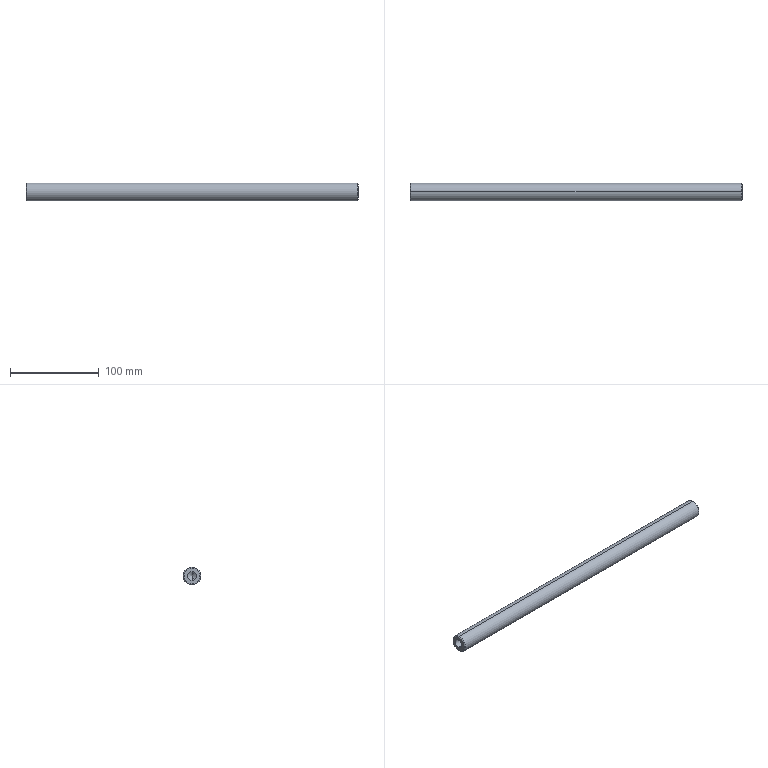Part | STEP file | BU-A02a | 1 solid | 16 faces | box 375 x 20 x 20 mm | volume 113660 mm3 | cone 8 | cylinder 6 | plane 2 | commonest cylinder face diameters 10.2 x4 20 x2
STEP:
#1=CARTESIAN_POINT('',(0.,0.,0.));
#2=DIRECTION('',(0.,0.,1.));
#3=DIRECTION('',(1.,0.,0.));
#4=AXIS2_PLACEMENT_3D('',#1,#2,#3);
#5=CARTESIAN_POINT('',(375.,0.,-9.));
#6=VERTEX_POINT('',#5);
#7=CARTESIAN_POINT('',(375.,0.,9.));
#8=VERTEX_POINT('',#7);
#9=CARTESIAN_POINT('',(375.,0.,0.));
#10=DIRECTION('',(1.,0.,0.));
#11=DIRECTION('',(0.,0.,1.));
#12=AXIS2_PLACEMENT_3D('',#9,#10,#11);
#13=CIRCLE('',#12,9.);
#14=CARTESIAN_POINT('',(374.,0.,0.));
#15=DIRECTION('',(-1.,0.,0.));
#16=DIRECTION('',(0.,0.,1.));
#17=AXIS2_PLACEMENT_3D('',#14,#15,#16);
#18=CONICAL_SURFACE('',#17,10.,0.7854);
#19=CARTESIAN_POINT('',(6.283,-1.));
#20=DIRECTION('',(-1.,0.));
#21=VECTOR('',#20,1.);
#22=LINE('',#19,#21);
#23=(GEOMETRIC_REPRESENTATION_CONTEXT(2)PARAMETRIC_REPRESENTATION_CONTEXT()REPRESENTATION_CONTEXT('',''));
#24=DEFINITIONAL_REPRESENTATION('',(#22),#23);
#25=PCURVE('',#18,#24);
#26=CARTESIAN_POINT('',(375.,0.,0.));
#27=DIRECTION('',(-1.,0.,0.));
#28=DIRECTION('',(0.,0.,1.));
#29=AXIS2_PLACEMENT_3D('',#26,#27,#28);
#30=PLANE('',#29);
#31=CARTESIAN_POINT('',(9.,0.));
#32=CARTESIAN_POINT('',(9.,-15.588));
#33=CARTESIAN_POINT('',(-4.5,-7.794));
#34=CARTESIAN_POINT('',(-18.,0.));
#35=CARTESIAN_POINT('',(-4.5,7.794));
#36=CARTESIAN_POINT('',(9.,15.588));
#37=CARTESIAN_POINT('',(9.,0.));
#38=(BOUNDED_CURVE()B_SPLINE_CURVE(2,(#31,#32,#33,#34,#35,#36,#37),.UNSPECIFIED.,.T.,.F.)B_SPLINE_CURVE_WITH_KNOTS((1,2,2,2,2,1),(-2.094,0.,2.094,4.189,6.283,8.378),.UNSPECIFIED.)CURVE()GEOMETRIC_REPRESENTATION_ITEM()RATIONAL_B_SPLINE_CURVE((1.,0.5,1.,0.5,1.,0.5,1.))REPRESENTATION_ITEM(''));
#39=(GEOMETRIC_REPRESENTATION_CONTEXT(2)PARAMETRIC_REPRESENTATION_CONTEXT()REPRESENTATION_CONTEXT('',''));
#40=DEFINITIONAL_REPRESENTATION('',(#38),#39);
#41=PCURVE('',#30,#40);
#42=SURFACE_CURVE('',#13,(#25,#41),.PCURVE_S1.);
#43=EDGE_CURVE('',#6,#8,#42,.T.);
#44=ORIENTED_EDGE('',*,*,#43,.F.);
#45=CARTESIAN_POINT('',(374.,0.,-10.));
#46=VERTEX_POINT('',#45);
#47=CARTESIAN_POINT('',(374.,0.,-10.));
#48=DIRECTION('',(-0.7071,0.,-0.7071));
#49=VECTOR('',#48,1.);
#50=LINE('',#47,#49);
#51=CARTESIAN_POINT('',(3.142,0.));
#52=DIRECTION('',(0.,1.));
#53=VECTOR('',#52,1.);
#54=LINE('',#51,#53);
#55=(GEOMETRIC_REPRESENTATION_CONTEXT(2)PARAMETRIC_REPRESENTATION_CONTEXT()REPRESENTATION_CONTEXT('',''));
#56=DEFINITIONAL_REPRESENTATION('',(#54),#55);
#57=PCURVE('',#18,#56);
#58=CARTESIAN_POINT('',(374.,0.,0.));
#59=DIRECTION('',(-1.,0.,0.));
#60=DIRECTION('',(0.,0.,1.));
#61=AXIS2_PLACEMENT_3D('',#58,#59,#60);
#62=CONICAL_SURFACE('',#61,10.,0.7854);
#63=CARTESIAN_POINT('',(3.142,0.));
#64=DIRECTION('',(0.,1.));
#65=VECTOR('',#64,1.);
#66=LINE('',#63,#65);
#67=(GEOMETRIC_REPRESENTATION_CONTEXT(2)PARAMETRIC_REPRESENTATION_CONTEXT()REPRESENTATION_CONTEXT('',''));
#68=DEFINITIONAL_REPRESENTATION('',(#66),#67);
#69=PCURVE('',#62,#68);
#70=SURFACE_CURVE('',#50,(#57,#69),.PCURVE_S1.);
#71=EDGE_CURVE('',#6,#46,#70,.T.);
#72=ORIENTED_EDGE('',*,*,#71,.T.);
#73=CARTESIAN_POINT('',(374.,0.,10.));
#74=VERTEX_POINT('',#73);
#75=CARTESIAN_POINT('',(374.,0.,0.));
#76=DIRECTION('',(-1.,0.,0.));
#77=DIRECTION('',(0.,0.,1.));
#78=AXIS2_PLACEMENT_3D('',#75,#76,#77);
#79=CIRCLE('',#78,10.);
#80=CARTESIAN_POINT('',(0.,0.));
#81=DIRECTION('',(1.,0.));
#82=VECTOR('',#81,1.);
#83=LINE('',#80,#82);
#84=(GEOMETRIC_REPRESENTATION_CONTEXT(2)PARAMETRIC_REPRESENTATION_CONTEXT()REPRESENTATION_CONTEXT('',''));
#85=DEFINITIONAL_REPRESENTATION('',(#83),#84);
#86=PCURVE('',#18,#85);
#87=CARTESIAN_POINT('',(-1000.,0.,0.));
#88=DIRECTION('',(-1.,0.,0.));
#89=DIRECTION('',(0.,0.,1.));
#90=AXIS2_PLACEMENT_3D('',#87,#88,#89);
#91=CYLINDRICAL_SURFACE('',#90,10.);
#92=CARTESIAN_POINT('',(0.,-1374.));
#93=DIRECTION('',(1.,0.));
#94=VECTOR('',#93,1.);
#95=LINE('',#92,#94);
#96=(GEOMETRIC_REPRESENTATION_CONTEXT(2)PARAMETRIC_REPRESENTATION_CONTEXT()REPRESENTATION_CONTEXT('',''));
#97=DEFINITIONAL_REPRESENTATION('',(#95),#96);
#98=PCURVE('',#91,#97);
#99=SURFACE_CURVE('',#79,(#86,#98),.PCURVE_S1.);
#100=EDGE_CURVE('',#74,#46,#99,.T.);
#101=ORIENTED_EDGE('',*,*,#100,.F.);
#102=CARTESIAN_POINT('',(374.,0.,10.));
#103=DIRECTION('',(-0.7071,0.,0.7071));
#104=VECTOR('',#103,1.);
#105=LINE('',#102,#104);
#106=CARTESIAN_POINT('',(0.,0.));
#107=DIRECTION('',(0.,1.));
#108=VECTOR('',#107,1.);
#109=LINE('',#106,#108);
#110=(GEOMETRIC_REPRESENTATION_CONTEXT(2)PARAMETRIC_REPRESENTATION_CONTEXT()REPRESENTATION_CONTEXT('',''));
#111=DEFINITIONAL_REPRESENTATION('',(#109),#110);
#112=PCURVE('',#18,#111);
#113=CARTESIAN_POINT('',(6.283,0.));
#114=DIRECTION('',(0.,1.));
#115=VECTOR('',#114,1.);
#116=LINE('',#113,#115);
#117=(GEOMETRIC_REPRESENTATION_CONTEXT(2)PARAMETRIC_REPRESENTATION_CONTEXT()REPRESENTATION_CONTEXT('',''));
#118=DEFINITIONAL_REPRESENTATION('',(#116),#117);
#119=PCURVE('',#62,#118);
#120=SURFACE_CURVE('',#105,(#112,#119),.PCURVE_S1.);
#121=EDGE_CURVE('',#8,#74,#120,.T.);
#122=ORIENTED_EDGE('',*,*,#121,.F.);
#123=EDGE_LOOP('',(#44,#72,#101,#122));
#124=FACE_BOUND('',#123,.T.);
#125=ADVANCED_FACE('',(#124),#18,.T.);
#126=CARTESIAN_POINT('',(0.,0.,9.));
#127=VERTEX_POINT('',#126);
#128=CARTESIAN_POINT('',(0.,0.,-9.));
#129=VERTEX_POINT('',#128);
#130=CARTESIAN_POINT('',(0.,0.,0.));
#131=DIRECTION('',(-1.,0.,0.));
#132=DIRECTION('',(0.,0.,-1.));
#133=AXIS2_PLACEMENT_3D('',#130,#131,#132);
#134=CIRCLE('',#133,9.);
#135=CARTESIAN_POINT('',(0.,0.,0.));
#136=DIRECTION('',(1.,0.,0.));
#137=DIRECTION('',(0.,0.,-1.));
#138=AXIS2_PLACEMENT_3D('',#135,#136,#137);
#139=CONICAL_SURFACE('',#138,9.,0.7854);
#140=CARTESIAN_POINT('',(6.283,0.));
#141=DIRECTION('',(-1.,0.));
#142=VECTOR('',#141,1.);
#143=LINE('',#140,#142);
#144=(GEOMETRIC_REPRESENTATION_CONTEXT(2)PARAMETRIC_REPRESENTATION_CONTEXT()REPRESENTATION_CONTEXT('',''));
#145=DEFINITIONAL_REPRESENTATION('',(#143),#144);
#146=PCURVE('',#139,#145);
#147=CARTESIAN_POINT('',(0.,0.,0.));
#148=DIRECTION('',(1.,0.,0.));
#149=DIRECTION('',(0.,0.,-1.));
#150=AXIS2_PLACEMENT_3D('',#147,#148,#149);
#151=PLANE('',#150);
#152=CARTESIAN_POINT('',(9.,0.));
#153=CARTESIAN_POINT('',(9.,-15.588));
#154=CARTESIAN_POINT('',(-4.5,-7.794));
#155=CARTESIAN_POINT('',(-18.,0.));
#156=CARTESIAN_POINT('',(-4.5,7.794));
#157=CARTESIAN_POINT('',(9.,15.588));
#158=CARTESIAN_POINT('',(9.,0.));
#159=(BOUNDED_CURVE()B_SPLINE_CURVE(2,(#152,#153,#154,#155,#156,#157,#158),.UNSPECIFIED.,.T.,.F.)B_SPLINE_CURVE_WITH_KNOTS((1,2,2,2,2,1),(-2.094,0.,2.094,4.189,6.283,8.378),.UNSPECIFIED.)CURVE()GEOMETRIC_REPRESENTATION_ITEM()RATIONAL_B_SPLINE_CURVE((1.,0.5,1.,0.5,1.,0.5,1.))REPRESENTATION_ITEM(''));
#160=(GEOMETRIC_REPRESENTATION_CONTEXT(2)PARAMETRIC_REPRESENTATION_CONTEXT()REPRESENTATION_CONTEXT('',''));
#161=DEFINITIONAL_REPRESENTATION('',(#159),#160);
#162=PCURVE('',#151,#161);
#163=SURFACE_CURVE('',#134,(#146,#162),.PCURVE_S1.);
#164=EDGE_CURVE('',#127,#129,#163,.T.);
#165=ORIENTED_EDGE('',*,*,#164,.F.);
#166=CARTESIAN_POINT('',(1.,0.,10.));
#167=VERTEX_POINT('',#166);
#168=CARTESIAN_POINT('',(0.,0.,9.));
#169=DIRECTION('',(0.7071,0.,0.7071));
#170=VECTOR('',#169,1.);
#171=LINE('',#168,#170);
#172=CARTESIAN_POINT('',(3.142,0.));
#173=DIRECTION('',(0.,1.));
#174=VECTOR('',#173,1.);
#175=LINE('',#172,#174);
#176=(GEOMETRIC_REPRESENTATION_CONTEXT(2)PARAMETRIC_REPRESENTATION_CONTEXT()REPRESENTATION_CONTEXT('',''));
#177=DEFINITIONAL_REPRESENTATION('',(#175),#176);
#178=PCURVE('',#139,#177);
#179=CARTESIAN_POINT('',(0.,0.,0.));
#180=DIRECTION('',(1.,0.,0.));
#181=DIRECTION('',(0.,0.,-1.));
#182=AXIS2_PLACEMENT_3D('',#179,#180,#181);
#183=CONICAL_SURFACE('',#182,9.,0.7854);
#184=CARTESIAN_POINT('',(3.142,0.));
#185=DIRECTION('',(0.,1.));
#186=VECTOR('',#185,1.);
#187=LINE('',#184,#186);
#188=(GEOMETRIC_REPRESENTATION_CONTEXT(2)PARAMETRIC_REPRESENTATION_CONTEXT()REPRESENTATION_CONTEXT('',''));
#189=DEFINITIONAL_REPRESENTATION('',(#187),#188);
#190=PCURVE('',#183,#189);
#191=SURFACE_CURVE('',#171,(#178,#190),.PCURVE_S1.);
#192=EDGE_CURVE('',#127,#167,#191,.T.);
#193=ORIENTED_EDGE('',*,*,#192,.T.);
#194=CARTESIAN_POINT('',(1.,0.,-10.));
#195=VERTEX_POINT('',#194);
#196=CARTESIAN_POINT('',(1.,0.,0.));
#197=DIRECTION('',(1.,0.,0.));
#198=DIRECTION('',(0.,0.,-1.));
#199=AXIS2_PLACEMENT_3D('',#196,#197,#198);
#200=CIRCLE('',#199,10.);
#201=CARTESIAN_POINT('',(0.,1.));
#202=DIRECTION('',(1.,0.));
#203=VECTOR('',#202,1.);
#204=LINE('',#201,#203);
#205=(GEOMETRIC_REPRESENTATION_CONTEXT(2)PARAMETRIC_REPRESENTATION_CONTEXT()REPRESENTATION_CONTEXT('',''));
#206=DEFINITIONAL_REPRESENTATION('',(#204),#205);
#207=PCURVE('',#139,#206);
#208=CARTESIAN_POINT('',(3.142,-1001.));
#209=DIRECTION('',(-1.,0.));
#210=VECTOR('',#209,1.);
#211=LINE('',#208,#210);
#212=(GEOMETRIC_REPRESENTATION_CONTEXT(2)PARAMETRIC_REPRESENTATION_CONTEXT()REPRESENTATION_CONTEXT('',''));
#213=DEFINITIONAL_REPRESENTATION('',(#211),#212);
#214=PCURVE('',#91,#213);
#215=SURFACE_CURVE('',#200,(#207,#214),.PCURVE_S1.);
#216=EDGE_CURVE('',#195,#167,#215,.T.);
#217=ORIENTED_EDGE('',*,*,#216,.F.);
#218=CARTESIAN_POINT('',(0.,0.,-9.));
#219=DIRECTION('',(0.7071,0.,-0.7071));
#220=VECTOR('',#219,1.);
#221=LINE('',#218,#220);
#222=CARTESIAN_POINT('',(0.,0.));
#223=DIRECTION('',(0.,1.));
#224=VECTOR('',#223,1.);
#225=LINE('',#222,#224);
#226=(GEOMETRIC_REPRESENTATION_CONTEXT(2)PARAMETRIC_REPRESENTATION_CONTEXT()REPRESENTATION_CONTEXT('',''));
#227=DEFINITIONAL_REPRESENTATION('',(#225),#226);
#228=PCURVE('',#139,#227);
#229=CARTESIAN_POINT('',(6.283,0.));
#230=DIRECTION('',(0.,1.));
#231=VECTOR('',#230,1.);
#232=LINE('',#229,#231);
#233=(GEOMETRIC_REPRESENTATION_CONTEXT(2)PARAMETRIC_REPRESENTATION_CONTEXT()REPRESENTATION_CONTEXT('',''));
#234=DEFINITIONAL_REPRESENTATION('',(#232),#233);
#235=PCURVE('',#183,#234);
#236=SURFACE_CURVE('',#221,(#228,#235),.PCURVE_S1.);
#237=EDGE_CURVE('',#129,#195,#236,.T.);
#238=ORIENTED_EDGE('',*,*,#237,.F.);
#239=EDGE_LOOP('',(#165,#193,#217,#238));
#240=FACE_BOUND('',#239,.T.);
#241=ADVANCED_FACE('',(#240),#139,.T.);
#242=CARTESIAN_POINT('',(24.,0.,-5.1));
#243=VERTEX_POINT('',#242);
#244=CARTESIAN_POINT('',(24.,0.,5.1));
#245=VERTEX_POINT('',#244);
#246=CARTESIAN_POINT('',(24.,0.,0.));
#247=DIRECTION('',(-1.,0.,0.));
#248=DIRECTION('',(0.,0.,1.));
#249=AXIS2_PLACEMENT_3D('',#246,#247,#248);
#250=CIRCLE('',#249,5.1);
#251=CARTESIAN_POINT('',(24.,0.,0.));
#252=DIRECTION('',(-1.,0.,0.));
#253=DIRECTION('',(0.,0.,1.));
#254=AXIS2_PLACEMENT_3D('',#251,#252,#253);
#255=CONICAL_SURFACE('',#254,5.1,1.03);
#256=CARTESIAN_POINT('',(0.,0.));
#257=DIRECTION('',(1.,0.));
#258=VECTOR('',#257,1.);
#259=LINE('',#256,#258);
#260=(GEOMETRIC_REPRESENTATION_CONTEXT(2)PARAMETRIC_REPRESENTATION_CONTEXT()REPRESENTATION_CONTEXT('',''));
#261=DEFINITIONAL_REPRESENTATION('',(#259),#260);
#262=PCURVE('',#255,#261);
#263=CARTESIAN_POINT('',(0.,0.,0.));
#264=DIRECTION('',(-1.,0.,0.));
#265=DIRECTION('',(0.,0.,1.));
#266=AXIS2_PLACEMENT_3D('',#263,#264,#265);
#267=CYLINDRICAL_SURFACE('',#266,5.1);
#268=CARTESIAN_POINT('',(0.,-24.));
#269=DIRECTION('',(1.,0.));
#270=VECTOR('',#269,1.);
#271=LINE('',#268,#270);
#272=(GEOMETRIC_REPRESENTATION_CONTEXT(2)PARAMETRIC_REPRESENTATION_CONTEXT()REPRESENTATION_CONTEXT('',''));
#273=DEFINITIONAL_REPRESENTATION('',(#271),#272);
#274=PCURVE('',#267,#273);
#275=SURFACE_CURVE('',#250,(#262,#274),.PCURVE_S1.);
#276=EDGE_CURVE('',#243,#245,#275,.T.);
#277=ORIENTED_EDGE('',*,*,#276,.F.);
#278=CARTESIAN_POINT('',(27.064,0.,0.));
#279=VERTEX_POINT('',#278);
#280=CARTESIAN_POINT('',(24.,0.,-5.1));
#281=DIRECTION('',(-0.515,0.,-0.8572));
#282=VECTOR('',#281,1.);
#283=LINE('',#280,#282);
#284=CARTESIAN_POINT('',(3.142,-3.064));
#285=CARTESIAN_POINT('',(3.142,-3.018));
#286=CARTESIAN_POINT('',(3.142,-2.925));
#287=CARTESIAN_POINT('',(3.142,-2.786));
#288=CARTESIAN_POINT('',(3.142,-2.647));
#289=CARTESIAN_POINT('',(3.142,-2.507));
#290=CARTESIAN_POINT('',(3.142,-2.368));
#291=CARTESIAN_POINT('',(3.142,-2.229));
#292=CARTESIAN_POINT('',(3.142,-2.089));
#293=CARTESIAN_POINT('',(3.142,-1.95));
#294=CARTESIAN_POINT('',(3.142,-1.811));
#295=CARTESIAN_POINT('',(3.142,-1.671));
#296=CARTESIAN_POINT('',(3.142,-1.532));
#297=CARTESIAN_POINT('',(3.142,-1.393));
#298=CARTESIAN_POINT('',(3.142,-1.254));
#299=CARTESIAN_POINT('',(3.142,-1.114));
#300=CARTESIAN_POINT('',(3.142,-0.975));
#301=CARTESIAN_POINT('',(3.142,-0.8357));
#302=CARTESIAN_POINT('',(3.142,-0.6965));
#303=CARTESIAN_POINT('',(3.142,-0.5572));
#304=CARTESIAN_POINT('',(3.142,-0.4179));
#305=CARTESIAN_POINT('',(3.142,-0.2786));
#306=CARTESIAN_POINT('',(3.142,-0.1393));
#307=CARTESIAN_POINT('',(3.142,-0.04643));
#308=CARTESIAN_POINT('',(3.142,0.));
#309=B_SPLINE_CURVE_WITH_KNOTS('',3,(#284,#285,#286,#287,#288,#289,#290,#291,#292,#293,#294,#295,#296,#297,#298,#299,#300,#301,#302,#303,#304,#305,#306,#307,#308),.UNSPECIFIED.,.F.,.F.,(4,1,1,1,1,1,1,1,1,1,1,1,1,1,1,1,1,1,1,1,1,1,4),(-5.95,-5.679,-5.409,-5.138,-4.868,-4.598,-4.327,-4.057,-3.786,-3.516,-3.245,-2.975,-2.704,-2.434,-2.164,-1.893,-1.623,-1.352,-1.082,-0.8113,-0.5409,-0.2704,0.),.QUASI_UNIFORM_KNOTS.);
#310=(GEOMETRIC_REPRESENTATION_CONTEXT(2)PARAMETRIC_REPRESENTATION_CONTEXT()REPRESENTATION_CONTEXT('',''));
#311=DEFINITIONAL_REPRESENTATION('',(#309),#310);
#312=PCURVE('',#255,#311);
#313=CARTESIAN_POINT('',(24.,0.,0.));
#314=DIRECTION('',(-1.,0.,0.));
#315=DIRECTION('',(0.,0.,1.));
#316=AXIS2_PLACEMENT_3D('',#313,#314,#315);
#317=CONICAL_SURFACE('',#316,5.1,1.03);
#318=CARTESIAN_POINT('',(3.142,-3.064));
#319=CARTESIAN_POINT('',(3.142,-3.018));
#320=CARTESIAN_POINT('',(3.142,-2.925));
#321=CARTESIAN_POINT('',(3.142,-2.786));
#322=CARTESIAN_POINT('',(3.142,-2.647));
#323=CARTESIAN_POINT('',(3.142,-2.507));
#324=CARTESIAN_POINT('',(3.142,-2.368));
#325=CARTESIAN_POINT('',(3.142,-2.229));
#326=CARTESIAN_POINT('',(3.142,-2.089));
#327=CARTESIAN_POINT('',(3.142,-1.95));
#328=CARTESIAN_POINT('',(3.142,-1.811));
#329=CARTESIAN_POINT('',(3.142,-1.671));
#330=CARTESIAN_POINT('',(3.142,-1.532));
#331=CARTESIAN_POINT('',(3.142,-1.393));
#332=CARTESIAN_POINT('',(3.142,-1.254));
#333=CARTESIAN_POINT('',(3.142,-1.114));
#334=CARTESIAN_POINT('',(3.142,-0.975));
#335=CARTESIAN_POINT('',(3.142,-0.8357));
#336=CARTESIAN_POINT('',(3.142,-0.6965));
#337=CARTESIAN_POINT('',(3.142,-0.5572));
#338=CARTESIAN_POINT('',(3.142,-0.4179));
#339=CARTESIAN_POINT('',(3.142,-0.2786));
#340=CARTESIAN_POINT('',(3.142,-0.1393));
#341=CARTESIAN_POINT('',(3.142,-0.04643));
#342=CARTESIAN_POINT('',(3.142,0.));
#343=B_SPLINE_CURVE_WITH_KNOTS('',3,(#318,#319,#320,#321,#322,#323,#324,#325,#326,#327,#328,#329,#330,#331,#332,#333,#334,#335,#336,#337,#338,#339,#340,#341,#342),.UNSPECIFIED.,.F.,.F.,(4,1,1,1,1,1,1,1,1,1,1,1,1,1,1,1,1,1,1,1,1,1,4),(-5.95,-5.679,-5.409,-5.138,-4.868,-4.598,-4.327,-4.057,-3.786,-3.516,-3.245,-2.975,-2.704,-2.434,-2.164,-1.893,-1.623,-1.352,-1.082,-0.8113,-0.5409,-0.2704,0.),.QUASI_UNIFORM_KNOTS.);
#344=(GEOMETRIC_REPRESENTATION_CONTEXT(2)PARAMETRIC_REPRESENTATION_CONTEXT()REPRESENTATION_CONTEXT('',''));
#345=DEFINITIONAL_REPRESENTATION('',(#343),#344);
#346=PCURVE('',#317,#345);
#347=SURFACE_CURVE('',#283,(#312,#346),.PCURVE_S1.);
#348=EDGE_CURVE('',#279,#243,#347,.T.);
#349=ORIENTED_EDGE('',*,*,#348,.F.);
#350=CARTESIAN_POINT('',(24.,0.,5.1));
#351=DIRECTION('',(-0.515,0.,0.8572));
#352=VECTOR('',#351,1.);
#353=LINE('',#350,#352);
#354=CARTESIAN_POINT('',(6.283,-3.064));
#355=CARTESIAN_POINT('',(6.283,-3.018));
#356=CARTESIAN_POINT('',(6.283,-2.925));
#357=CARTESIAN_POINT('',(6.283,-2.786));
#358=CARTESIAN_POINT('',(6.283,-2.647));
#359=CARTESIAN_POINT('',(6.283,-2.507));
#360=CARTESIAN_POINT('',(6.283,-2.368));
#361=CARTESIAN_POINT('',(6.283,-2.229));
#362=CARTESIAN_POINT('',(6.283,-2.089));
#363=CARTESIAN_POINT('',(6.283,-1.95));
#364=CARTESIAN_POINT('',(6.283,-1.811));
#365=CARTESIAN_POINT('',(6.283,-1.671));
#366=CARTESIAN_POINT('',(6.283,-1.532));
#367=CARTESIAN_POINT('',(6.283,-1.393));
#368=CARTESIAN_POINT('',(6.283,-1.254));
#369=CARTESIAN_POINT('',(6.283,-1.114));
#370=CARTESIAN_POINT('',(6.283,-0.975));
#371=CARTESIAN_POINT('',(6.283,-0.8357));
#372=CARTESIAN_POINT('',(6.283,-0.6965));
#373=CARTESIAN_POINT('',(6.283,-0.5572));
#374=CARTESIAN_POINT('',(6.283,-0.4179));
#375=CARTESIAN_POINT('',(6.283,-0.2786));
#376=CARTESIAN_POINT('',(6.283,-0.1393));
#377=CARTESIAN_POINT('',(6.283,-0.04643));
#378=CARTESIAN_POINT('',(6.283,0.));
#379=B_SPLINE_CURVE_WITH_KNOTS('',3,(#354,#355,#356,#357,#358,#359,#360,#361,#362,#363,#364,#365,#366,#367,#368,#369,#370,#371,#372,#373,#374,#375,#376,#377,#378),.UNSPECIFIED.,.F.,.F.,(4,1,1,1,1,1,1,1,1,1,1,1,1,1,1,1,1,1,1,1,1,1,4),(-5.95,-5.679,-5.409,-5.138,-4.868,-4.598,-4.327,-4.057,-3.786,-3.516,-3.245,-2.975,-2.704,-2.434,-2.164,-1.893,-1.623,-1.352,-1.082,-0.8113,-0.5409,-0.2704,0.),.QUASI_UNIFORM_KNOTS.);
#380=(GEOMETRIC_REPRESENTATION_CONTEXT(2)PARAMETRIC_REPRESENTATION_CONTEXT()REPRESENTATION_CONTEXT('',''));
#381=DEFINITIONAL_REPRESENTATION('',(#379),#380);
#382=PCURVE('',#255,#381);
#383=CARTESIAN_POINT('',(0.,-3.064));
#384=CARTESIAN_POINT('',(0.,-3.018));
#385=CARTESIAN_POINT('',(0.,-2.925));
#386=CARTESIAN_POINT('',(0.,-2.786));
#387=CARTESIAN_POINT('',(0.,-2.647));
#388=CARTESIAN_POINT('',(0.,-2.507));
#389=CARTESIAN_POINT('',(0.,-2.368));
#390=CARTESIAN_POINT('',(0.,-2.229));
#391=CARTESIAN_POINT('',(0.,-2.089));
#392=CARTESIAN_POINT('',(0.,-1.95));
#393=CARTESIAN_POINT('',(0.,-1.811));
#394=CARTESIAN_POINT('',(0.,-1.671));
#395=CARTESIAN_POINT('',(0.,-1.532));
#396=CARTESIAN_POINT('',(0.,-1.393));
#397=CARTESIAN_POINT('',(0.,-1.254));
#398=CARTESIAN_POINT('',(0.,-1.114));
#399=CARTESIAN_POINT('',(0.,-0.975));
#400=CARTESIAN_POINT('',(0.,-0.8357));
#401=CARTESIAN_POINT('',(0.,-0.6965));
#402=CARTESIAN_POINT('',(0.,-0.5572));
#403=CARTESIAN_POINT('',(0.,-0.4179));
#404=CARTESIAN_POINT('',(0.,-0.2786));
#405=CARTESIAN_POINT('',(0.,-0.1393));
#406=CARTESIAN_POINT('',(0.,-0.04643));
#407=CARTESIAN_POINT('',(0.,0.));
#408=B_SPLINE_CURVE_WITH_KNOTS('',3,(#383,#384,#385,#386,#387,#388,#389,#390,#391,#392,#393,#394,#395,#396,#397,#398,#399,#400,#401,#402,#403,#404,#405,#406,#407),.UNSPECIFIED.,.F.,.F.,(4,1,1,1,1,1,1,1,1,1,1,1,1,1,1,1,1,1,1,1,1,1,4),(-5.95,-5.679,-5.409,-5.138,-4.868,-4.598,-4.327,-4.057,-3.786,-3.516,-3.245,-2.975,-2.704,-2.434,-2.164,-1.893,-1.623,-1.352,-1.082,-0.8113,-0.5409,-0.2704,0.),.QUASI_UNIFORM_KNOTS.);
#409=(GEOMETRIC_REPRESENTATION_CONTEXT(2)PARAMETRIC_REPRESENTATION_CONTEXT()REPRESENTATION_CONTEXT('',''));
#410=DEFINITIONAL_REPRESENTATION('',(#408),#409);
#411=PCURVE('',#317,#410);
#412=SURFACE_CURVE('',#353,(#382,#411),.PCURVE_S1.);
#413=EDGE_CURVE('',#279,#245,#412,.T.);
#414=ORIENTED_EDGE('',*,*,#413,.T.);
#415=EDGE_LOOP('',(#277,#349,#414));
#416=FACE_BOUND('',#415,.F.);
#417=ADVANCED_FACE('',(#416),#255,.F.);
#418=CARTESIAN_POINT('',(0.,0.,5.1));
#419=VERTEX_POINT('',#418);
#420=CARTESIAN_POINT('',(0.,0.,5.1));
#421=DIRECTION('',(-1.,0.,0.));
#422=VECTOR('',#421,1.);
#423=LINE('',#420,#422);
#424=CARTESIAN_POINT('',(6.283,0.));
#425=DIRECTION('',(0.,1.));
#426=VECTOR('',#425,1.);
#427=LINE('',#424,#426);
#428=(GEOMETRIC_REPRESENTATION_CONTEXT(2)PARAMETRIC_REPRESENTATION_CONTEXT()REPRESENTATION_CONTEXT('',''));
#429=DEFINITIONAL_REPRESENTATION('',(#427),#428);
#430=PCURVE('',#267,#429);
#431=CARTESIAN_POINT('',(0.,0.,0.));
#432=DIRECTION('',(-1.,0.,0.));
#433=DIRECTION('',(0.,0.,1.));
#434=AXIS2_PLACEMENT_3D('',#431,#432,#433);
#435=CYLINDRICAL_SURFACE('',#434,5.1);
#436=CARTESIAN_POINT('',(0.,0.));
#437=DIRECTION('',(0.,1.));
#438=VECTOR('',#437,1.);
#439=LINE('',#436,#438);
#440=(GEOMETRIC_REPRESENTATION_CONTEXT(2)PARAMETRIC_REPRESENTATION_CONTEXT()REPRESENTATION_CONTEXT('',''));
#441=DEFINITIONAL_REPRESENTATION('',(#439),#440);
#442=PCURVE('',#435,#441);
#443=SURFACE_CURVE('',#423,(#430,#442),.PCURVE_S1.);
#444=EDGE_CURVE('',#245,#419,#443,.T.);
#445=ORIENTED_EDGE('',*,*,#444,.T.);
#446=CARTESIAN_POINT('',(0.,0.,-5.1));
#447=VERTEX_POINT('',#446);
#448=CARTESIAN_POINT('',(0.,0.,0.));
#449=DIRECTION('',(-1.,0.,0.));
#450=DIRECTION('',(0.,0.,1.));
#451=AXIS2_PLACEMENT_3D('',#448,#449,#450);
#452=CIRCLE('',#451,5.1);
#453=CARTESIAN_POINT('',(0.,0.));
#454=DIRECTION('',(1.,0.));
#455=VECTOR('',#454,1.);
#456=LINE('',#453,#455);
#457=(GEOMETRIC_REPRESENTATION_CONTEXT(2)PARAMETRIC_REPRESENTATION_CONTEXT()REPRESENTATION_CONTEXT('',''));
#458=DEFINITIONAL_REPRESENTATION('',(#456),#457);
#459=PCURVE('',#267,#458);
#460=CARTESIAN_POINT('',(-5.1,0.));
#461=CARTESIAN_POINT('',(-5.1,8.833));
#462=CARTESIAN_POINT('',(2.55,4.417));
#463=CARTESIAN_POINT('',(10.2,0.));
#464=CARTESIAN_POINT('',(2.55,-4.417));
#465=CARTESIAN_POINT('',(-5.1,-8.833));
#466=CARTESIAN_POINT('',(-5.1,0.));
#467=(BOUNDED_CURVE()B_SPLINE_CURVE(2,(#460,#461,#462,#463,#464,#465,#466),.UNSPECIFIED.,.T.,.F.)B_SPLINE_CURVE_WITH_KNOTS((1,2,2,2,2,1),(-2.094,0.,2.094,4.189,6.283,8.378),.UNSPECIFIED.)CURVE()GEOMETRIC_REPRESENTATION_ITEM()RATIONAL_B_SPLINE_CURVE((1.,0.5,1.,0.5,1.,0.5,1.))REPRESENTATION_ITEM(''));
#468=(GEOMETRIC_REPRESENTATION_CONTEXT(2)PARAMETRIC_REPRESENTATION_CONTEXT()REPRESENTATION_CONTEXT('',''));
#469=DEFINITIONAL_REPRESENTATION('',(#467),#468);
#470=PCURVE('',#151,#469);
#471=SURFACE_CURVE('',#452,(#459,#470),.PCURVE_S1.);
#472=EDGE_CURVE('',#447,#419,#471,.T.);
#473=ORIENTED_EDGE('',*,*,#472,.F.);
#474=CARTESIAN_POINT('',(0.,0.,-5.1));
#475=DIRECTION('',(-1.,0.,0.));
#476=VECTOR('',#475,1.);
#477=LINE('',#474,#476);
#478=CARTESIAN_POINT('',(3.142,0.));
#479=DIRECTION('',(0.,1.));
#480=VECTOR('',#479,1.);
#481=LINE('',#478,#480);
#482=(GEOMETRIC_REPRESENTATION_CONTEXT(2)PARAMETRIC_REPRESENTATION_CONTEXT()REPRESENTATION_CONTEXT('',''));
#483=DEFINITIONAL_REPRESENTATION('',(#481),#482);
#484=PCURVE('',#267,#483);
#485=CARTESIAN_POINT('',(3.142,0.));
#486=DIRECTION('',(0.,1.));
#487=VECTOR('',#486,1.);
#488=LINE('',#485,#487);
#489=(GEOMETRIC_REPRESENTATION_CONTEXT(2)PARAMETRIC_REPRESENTATION_CONTEXT()REPRESENTATION_CONTEXT('',''));
#490=DEFINITIONAL_REPRESENTATION('',(#488),#489);
#491=PCURVE('',#435,#490);
#492=SURFACE_CURVE('',#477,(#484,#491),.PCURVE_S1.);
#493=EDGE_CURVE('',#243,#447,#492,.T.);
#494=ORIENTED_EDGE('',*,*,#493,.F.);
#495=ORIENTED_EDGE('',*,*,#276,.T.);
#496=EDGE_LOOP('',(#445,#473,#494,#495));
#497=FACE_BOUND('',#496,.F.);
#498=ADVANCED_FACE('',(#497),#267,.F.);
#499=CARTESIAN_POINT('',(351.,0.,5.1));
#500=VERTEX_POINT('',#499);
#501=CARTESIAN_POINT('',(351.,0.,-5.1));
#502=VERTEX_POINT('',#501);
#503=CARTESIAN_POINT('',(351.,0.,0.));
#504=DIRECTION('',(1.,0.,0.));
#505=DIRECTION('',(0.,0.,-1.));
#506=AXIS2_PLACEMENT_3D('',#503,#504,#505);
#507=CIRCLE('',#506,5.1);
#508=CARTESIAN_POINT('',(351.,0.,0.));
#509=DIRECTION('',(1.,0.,0.));
#510=DIRECTION('',(0.,0.,-1.));
#511=AXIS2_PLACEMENT_3D('',#508,#509,#510);
#512=CONICAL_SURFACE('',#511,5.1,1.03);
#513=CARTESIAN_POINT('',(0.,0.));
#514=DIRECTION('',(1.,0.));
#515=VECTOR('',#514,1.);
#516=LINE('',#513,#515);
#517=(GEOMETRIC_REPRESENTATION_CONTEXT(2)PARAMETRIC_REPRESENTATION_CONTEXT()REPRESENTATION_CONTEXT('',''));
#518=DEFINITIONAL_REPRESENTATION('',(#516),#517);
#519=PCURVE('',#512,#518);
#520=CARTESIAN_POINT('',(375.,0.,0.));
#521=DIRECTION('',(1.,0.,0.));
#522=DIRECTION('',(0.,0.,-1.));
#523=AXIS2_PLACEMENT_3D('',#520,#521,#522);
#524=CYLINDRICAL_SURFACE('',#523,5.1);
#525=CARTESIAN_POINT('',(0.,-24.));
#526=DIRECTION('',(1.,0.));
#527=VECTOR('',#526,1.);
#528=LINE('',#525,#527);
#529=(GEOMETRIC_REPRESENTATION_CONTEXT(2)PARAMETRIC_REPRESENTATION_CONTEXT()REPRESENTATION_CONTEXT('',''));
#530=DEFINITIONAL_REPRESENTATION('',(#528),#529);
#531=PCURVE('',#524,#530);
#532=SURFACE_CURVE('',#507,(#519,#531),.PCURVE_S1.);
#533=EDGE_CURVE('',#500,#502,#532,.T.);
#534=ORIENTED_EDGE('',*,*,#533,.F.);
#535=CARTESIAN_POINT('',(347.936,0.,0.));
#536=VERTEX_POINT('',#535);
#537=CARTESIAN_POINT('',(351.,0.,5.1));
#538=DIRECTION('',(0.515,0.,0.8572));
#539=VECTOR('',#538,1.);
#540=LINE('',#537,#539);
#541=CARTESIAN_POINT('',(3.142,0.));
#542=DIRECTION('',(0.,1.));
#543=VECTOR('',#542,1.);
#544=LINE('',#541,#543);
#545=(GEOMETRIC_REPRESENTATION_CONTEXT(2)PARAMETRIC_REPRESENTATION_CONTEXT()REPRESENTATION_CONTEXT('',''));
#546=DEFINITIONAL_REPRESENTATION('',(#544),#545);
#547=PCURVE('',#512,#546);
#548=CARTESIAN_POINT('',(351.,0.,0.));
#549=DIRECTION('',(1.,0.,0.));
#550=DIRECTION('',(0.,0.,-1.));
#551=AXIS2_PLACEMENT_3D('',#548,#549,#550);
#552=CONICAL_SURFACE('',#551,5.1,1.03);
#553=CARTESIAN_POINT('',(3.142,0.));
#554=DIRECTION('',(0.,1.));
#555=VECTOR('',#554,1.);
#556=LINE('',#553,#555);
#557=(GEOMETRIC_REPRESENTATION_CONTEXT(2)PARAMETRIC_REPRESENTATION_CONTEXT()REPRESENTATION_CONTEXT('',''));
#558=DEFINITIONAL_REPRESENTATION('',(#556),#557);
#559=PCURVE('',#552,#558);
#560=SURFACE_CURVE('',#540,(#547,#559),.PCURVE_S1.);
#561=EDGE_CURVE('',#536,#500,#560,.T.);
#562=ORIENTED_EDGE('',*,*,#561,.F.);
#563=CARTESIAN_POINT('',(351.,0.,-5.1));
#564=DIRECTION('',(0.515,0.,-0.8572));
#565=VECTOR('',#564,1.);
#566=LINE('',#563,#565);
#567=CARTESIAN_POINT('',(6.283,0.));
#568=DIRECTION('',(0.,1.));
#569=VECTOR('',#568,1.);
#570=LINE('',#567,#569);
#571=(GEOMETRIC_REPRESENTATION_CONTEXT(2)PARAMETRIC_REPRESENTATION_CONTEXT()REPRESENTATION_CONTEXT('',''));
#572=DEFINITIONAL_REPRESENTATION('',(#570),#571);
#573=PCURVE('',#512,#572);
#574=CARTESIAN_POINT('',(0.,0.));
#575=DIRECTION('',(0.,1.));
#576=VECTOR('',#575,1.);
#577=LINE('',#574,#576);
#578=(GEOMETRIC_REPRESENTATION_CONTEXT(2)PARAMETRIC_REPRESENTATION_CONTEXT()REPRESENTATION_CONTEXT('',''));
#579=DEFINITIONAL_REPRESENTATION('',(#577),#578);
#580=PCURVE('',#552,#579);
#581=SURFACE_CURVE('',#566,(#573,#580),.PCURVE_S1.);
#582=EDGE_CURVE('',#536,#502,#581,.T.);
#583=ORIENTED_EDGE('',*,*,#582,.T.);
#584=EDGE_LOOP('',(#534,#562,#583));
#585=FACE_BOUND('',#584,.F.);
#586=ADVANCED_FACE('',(#585),#512,.F.);
#587=CARTESIAN_POINT('',(375.,0.,-5.1));
#588=VERTEX_POINT('',#587);
#589=CARTESIAN_POINT('',(375.,0.,-5.1));
#590=DIRECTION('',(1.,0.,0.));
#591=VECTOR('',#590,1.);
#592=LINE('',#589,#591);
#593=CARTESIAN_POINT('',(6.283,0.));
#594=DIRECTION('',(0.,1.));
#595=VECTOR('',#594,1.);
#596=LINE('',#593,#595);
#597=(GEOMETRIC_REPRESENTATION_CONTEXT(2)PARAMETRIC_REPRESENTATION_CONTEXT()REPRESENTATION_CONTEXT('',''));
#598=DEFINITIONAL_REPRESENTATION('',(#596),#597);
#599=PCURVE('',#524,#598);
#600=CARTESIAN_POINT('',(375.,0.,0.));
#601=DIRECTION('',(1.,0.,0.));
#602=DIRECTION('',(0.,0.,-1.));
#603=AXIS2_PLACEMENT_3D('',#600,#601,#602);
#604=CYLINDRICAL_SURFACE('',#603,5.1);
#605=CARTESIAN_POINT('',(0.,0.));
#606=DIRECTION('',(0.,1.));
#607=VECTOR('',#606,1.);
#608=LINE('',#605,#607);
#609=(GEOMETRIC_REPRESENTATION_CONTEXT(2)PARAMETRIC_REPRESENTATION_CONTEXT()REPRESENTATION_CONTEXT('',''));
#610=DEFINITIONAL_REPRESENTATION('',(#608),#609);
#611=PCURVE('',#604,#610);
#612=SURFACE_CURVE('',#592,(#599,#611),.PCURVE_S1.);
#613=EDGE_CURVE('',#502,#588,#612,.T.);
#614=ORIENTED_EDGE('',*,*,#613,.T.);
#615=CARTESIAN_POINT('',(375.,0.,5.1));
#616=VERTEX_POINT('',#615);
#617=CARTESIAN_POINT('',(375.,0.,0.));
#618=DIRECTION('',(1.,0.,0.));
#619=DIRECTION('',(0.,0.,-1.));
#620=AXIS2_PLACEMENT_3D('',#617,#618,#619);
#621=CIRCLE('',#620,5.1);
#622=CARTESIAN_POINT('',(0.,0.));
#623=DIRECTION('',(1.,0.));
#624=VECTOR('',#623,1.);
#625=LINE('',#622,#624);
#626=(GEOMETRIC_REPRESENTATION_CONTEXT(2)PARAMETRIC_REPRESENTATION_CONTEXT()REPRESENTATION_CONTEXT('',''));
#627=DEFINITIONAL_REPRESENTATION('',(#625),#626);
#628=PCURVE('',#524,#627);
#629=CARTESIAN_POINT('',(-5.1,0.));
#630=CARTESIAN_POINT('',(-5.1,8.833));
#631=CARTESIAN_POINT('',(2.55,4.417));
#632=CARTESIAN_POINT('',(10.2,0.));
#633=CARTESIAN_POINT('',(2.55,-4.417));
#634=CARTESIAN_POINT('',(-5.1,-8.833));
#635=CARTESIAN_POINT('',(-5.1,0.));
#636=(BOUNDED_CURVE()B_SPLINE_CURVE(2,(#629,#630,#631,#632,#633,#634,#635),.UNSPECIFIED.,.T.,.F.)B_SPLINE_CURVE_WITH_KNOTS((1,2,2,2,2,1),(-2.094,0.,2.094,4.189,6.283,8.378),.UNSPECIFIED.)CURVE()GEOMETRIC_REPRESENTATION_ITEM()RATIONAL_B_SPLINE_CURVE((1.,0.5,1.,0.5,1.,0.5,1.))REPRESENTATION_ITEM(''));
#637=(GEOMETRIC_REPRESENTATION_CONTEXT(2)PARAMETRIC_REPRESENTATION_CONTEXT()REPRESENTATION_CONTEXT('',''));
#638=DEFINITIONAL_REPRESENTATION('',(#636),#637);
#639=PCURVE('',#30,#638);
#640=SURFACE_CURVE('',#621,(#628,#639),.PCURVE_S1.);
#641=EDGE_CURVE('',#616,#588,#640,.T.);
#642=ORIENTED_EDGE('',*,*,#641,.F.);
#643=CARTESIAN_POINT('',(375.,0.,5.1));
#644=DIRECTION('',(1.,0.,0.));
#645=VECTOR('',#644,1.);
#646=LINE('',#643,#645);
#647=CARTESIAN_POINT('',(3.142,0.));
#648=DIRECTION('',(0.,1.));
#649=VECTOR('',#648,1.);
#650=LINE('',#647,#649);
#651=(GEOMETRIC_REPRESENTATION_CONTEXT(2)PARAMETRIC_REPRESENTATION_CONTEXT()REPRESENTATION_CONTEXT('',''));
#652=DEFINITIONAL_REPRESENTATION('',(#650),#651);
#653=PCURVE('',#524,#652);
#654=CARTESIAN_POINT('',(3.142,0.));
#655=DIRECTION('',(0.,1.));
#656=VECTOR('',#655,1.);
#657=LINE('',#654,#656);
#658=(GEOMETRIC_REPRESENTATION_CONTEXT(2)PARAMETRIC_REPRESENTATION_CONTEXT()REPRESENTATION_CONTEXT('',''));
#659=DEFINITIONAL_REPRESENTATION('',(#657),#658);
#660=PCURVE('',#604,#659);
#661=SURFACE_CURVE('',#646,(#653,#660),.PCURVE_S1.);
#662=EDGE_CURVE('',#500,#616,#661,.T.);
#663=ORIENTED_EDGE('',*,*,#662,.F.);
#664=ORIENTED_EDGE('',*,*,#533,.T.);
#665=EDGE_LOOP('',(#614,#642,#663,#664));
#666=FACE_BOUND('',#665,.F.);
#667=ADVANCED_FACE('',(#666),#524,.F.);
#668=ORIENTED_EDGE('',*,*,#100,.T.);
#669=CARTESIAN_POINT('',(-1000.,0.,-10.));
#670=DIRECTION('',(-1.,0.,0.));
#671=VECTOR('',#670,1.);
#672=LINE('',#669,#671);
#673=CARTESIAN_POINT('',(3.142,0.));
#674=DIRECTION('',(0.,1.));
#675=VECTOR('',#674,1.);
#676=LINE('',#673,#675);
#677=(GEOMETRIC_REPRESENTATION_CONTEXT(2)PARAMETRIC_REPRESENTATION_CONTEXT()REPRESENTATION_CONTEXT('',''));
#678=DEFINITIONAL_REPRESENTATION('',(#676),#677);
#679=PCURVE('',#91,#678);
#680=CARTESIAN_POINT('',(-1000.,0.,0.));
#681=DIRECTION('',(-1.,0.,0.));
#682=DIRECTION('',(0.,0.,1.));
#683=AXIS2_PLACEMENT_3D('',#680,#681,#682);
#684=CYLINDRICAL_SURFACE('',#683,10.);
#685=CARTESIAN_POINT('',(3.142,0.));
#686=DIRECTION('',(0.,1.));
#687=VECTOR('',#686,1.);
#688=LINE('',#685,#687);
#689=(GEOMETRIC_REPRESENTATION_CONTEXT(2)PARAMETRIC_REPRESENTATION_CONTEXT()REPRESENTATION_CONTEXT('',''));
#690=DEFINITIONAL_REPRESENTATION('',(#688),#689);
#691=PCURVE('',#684,#690);
#692=SURFACE_CURVE('',#672,(#679,#691),.PCURVE_S1.);
#693=EDGE_CURVE('',#46,#195,#692,.T.);
#694=ORIENTED_EDGE('',*,*,#693,.T.);
#695=ORIENTED_EDGE('',*,*,#216,.T.);
#696=CARTESIAN_POINT('',(-1000.,0.,10.));
#697=DIRECTION('',(-1.,0.,0.));
#698=VECTOR('',#697,1.);
#699=LINE('',#696,#698);
#700=CARTESIAN_POINT('',(0.,0.));
#701=DIRECTION('',(0.,1.));
#702=VECTOR('',#701,1.);
#703=LINE('',#700,#702);
#704=(GEOMETRIC_REPRESENTATION_CONTEXT(2)PARAMETRIC_REPRESENTATION_CONTEXT()REPRESENTATION_CONTEXT('',''));
#705=DEFINITIONAL_REPRESENTATION('',(#703),#704);
#706=PCURVE('',#91,#705);
#707=CARTESIAN_POINT('',(6.283,0.));
#708=DIRECTION('',(0.,1.));
#709=VECTOR('',#708,1.);
#710=LINE('',#707,#709);
#711=(GEOMETRIC_REPRESENTATION_CONTEXT(2)PARAMETRIC_REPRESENTATION_CONTEXT()REPRESENTATION_CONTEXT('',''));
#712=DEFINITIONAL_REPRESENTATION('',(#710),#711);
#713=PCURVE('',#684,#712);
#714=SURFACE_CURVE('',#699,(#706,#713),.PCURVE_S1.);
#715=EDGE_CURVE('',#74,#167,#714,.T.);
#716=ORIENTED_EDGE('',*,*,#715,.F.);
#717=EDGE_LOOP('',(#668,#694,#695,#716));
#718=FACE_BOUND('',#717,.T.);
#719=ADVANCED_FACE('',(#718),#91,.T.);
#720=CARTESIAN_POINT('',(0.,0.,0.));
#721=DIRECTION('',(-1.,0.,0.));
#722=DIRECTION('',(0.,0.,-1.));
#723=AXIS2_PLACEMENT_3D('',#720,#721,#722);
#724=CIRCLE('',#723,9.);
#725=CARTESIAN_POINT('',(9.,0.));
#726=CARTESIAN_POINT('',(9.,-15.588));
#727=CARTESIAN_POINT('',(-4.5,-7.794));
#728=CARTESIAN_POINT('',(-18.,0.));
#729=CARTESIAN_POINT('',(-4.5,7.794));
#730=CARTESIAN_POINT('',(9.,15.588));
#731=CARTESIAN_POINT('',(9.,0.));
#732=(BOUNDED_CURVE()B_SPLINE_CURVE(2,(#725,#726,#727,#728,#729,#730,#731),.UNSPECIFIED.,.T.,.F.)B_SPLINE_CURVE_WITH_KNOTS((1,2,2,2,2,1),(-2.094,0.,2.094,4.189,6.283,8.378),.UNSPECIFIED.)CURVE()GEOMETRIC_REPRESENTATION_ITEM()RATIONAL_B_SPLINE_CURVE((1.,0.5,1.,0.5,1.,0.5,1.))REPRESENTATION_ITEM(''));
#733=(GEOMETRIC_REPRESENTATION_CONTEXT(2)PARAMETRIC_REPRESENTATION_CONTEXT()REPRESENTATION_CONTEXT('',''));
#734=DEFINITIONAL_REPRESENTATION('',(#732),#733);
#735=PCURVE('',#151,#734);
#736=CARTESIAN_POINT('',(6.283,0.));
#737=DIRECTION('',(-1.,0.));
#738=VECTOR('',#737,1.);
#739=LINE('',#736,#738);
#740=(GEOMETRIC_REPRESENTATION_CONTEXT(2)PARAMETRIC_REPRESENTATION_CONTEXT()REPRESENTATION_CONTEXT('',''));
#741=DEFINITIONAL_REPRESENTATION('',(#739),#740);
#742=PCURVE('',#183,#741);
#743=SURFACE_CURVE('',#724,(#735,#742),.PCURVE_S1.);
#744=EDGE_CURVE('',#129,#127,#743,.T.);
#745=ORIENTED_EDGE('',*,*,#744,.T.);
#746=ORIENTED_EDGE('',*,*,#164,.T.);
#747=EDGE_LOOP('',(#745,#746));
#748=FACE_BOUND('',#747,.T.);
#749=CARTESIAN_POINT('',(0.,0.,0.));
#750=DIRECTION('',(-1.,0.,0.));
#751=DIRECTION('',(0.,0.,1.));
#752=AXIS2_PLACEMENT_3D('',#749,#750,#751);
#753=CIRCLE('',#752,5.1);
#754=CARTESIAN_POINT('',(-5.1,0.));
#755=CARTESIAN_POINT('',(-5.1,8.833));
#756=CARTESIAN_POINT('',(2.55,4.417));
#757=CARTESIAN_POINT('',(10.2,0.));
#758=CARTESIAN_POINT('',(2.55,-4.417));
#759=CARTESIAN_POINT('',(-5.1,-8.833));
#760=CARTESIAN_POINT('',(-5.1,0.));
#761=(BOUNDED_CURVE()B_SPLINE_CURVE(2,(#754,#755,#756,#757,#758,#759,#760),.UNSPECIFIED.,.T.,.F.)B_SPLINE_CURVE_WITH_KNOTS((1,2,2,2,2,1),(-2.094,0.,2.094,4.189,6.283,8.378),.UNSPECIFIED.)CURVE()GEOMETRIC_REPRESENTATION_ITEM()RATIONAL_B_SPLINE_CURVE((1.,0.5,1.,0.5,1.,0.5,1.))REPRESENTATION_ITEM(''));
#762=(GEOMETRIC_REPRESENTATION_CONTEXT(2)PARAMETRIC_REPRESENTATION_CONTEXT()REPRESENTATION_CONTEXT('',''));
#763=DEFINITIONAL_REPRESENTATION('',(#761),#762);
#764=PCURVE('',#151,#763);
#765=CARTESIAN_POINT('',(0.,0.));
#766=DIRECTION('',(1.,0.));
#767=VECTOR('',#766,1.);
#768=LINE('',#765,#767);
#769=(GEOMETRIC_REPRESENTATION_CONTEXT(2)PARAMETRIC_REPRESENTATION_CONTEXT()REPRESENTATION_CONTEXT('',''));
#770=DEFINITIONAL_REPRESENTATION('',(#768),#769);
#771=PCURVE('',#435,#770);
#772=SURFACE_CURVE('',#753,(#764,#771),.PCURVE_S1.);
#773=EDGE_CURVE('',#419,#447,#772,.T.);
#774=ORIENTED_EDGE('',*,*,#773,.F.);
#775=ORIENTED_EDGE('',*,*,#472,.F.);
#776=EDGE_LOOP('',(#774,#775));
#777=FACE_BOUND('',#776,.T.);
#778=ADVANCED_FACE('',(#748,#777),#151,.F.);
#779=ORIENTED_EDGE('',*,*,#693,.F.);
#780=CARTESIAN_POINT('',(374.,0.,0.));
#781=DIRECTION('',(-1.,0.,0.));
#782=DIRECTION('',(0.,0.,1.));
#783=AXIS2_PLACEMENT_3D('',#780,#781,#782);
#784=CIRCLE('',#783,10.);
#785=CARTESIAN_POINT('',(0.,-1374.));
#786=DIRECTION('',(1.,0.));
#787=VECTOR('',#786,1.);
#788=LINE('',#785,#787);
#789=(GEOMETRIC_REPRESENTATION_CONTEXT(2)PARAMETRIC_REPRESENTATION_CONTEXT()REPRESENTATION_CONTEXT('',''));
#790=DEFINITIONAL_REPRESENTATION('',(#788),#789);
#791=PCURVE('',#684,#790);
#792=CARTESIAN_POINT('',(0.,0.));
#793=DIRECTION('',(1.,0.));
#794=VECTOR('',#793,1.);
#795=LINE('',#792,#794);
#796=(GEOMETRIC_REPRESENTATION_CONTEXT(2)PARAMETRIC_REPRESENTATION_CONTEXT()REPRESENTATION_CONTEXT('',''));
#797=DEFINITIONAL_REPRESENTATION('',(#795),#796);
#798=PCURVE('',#62,#797);
#799=SURFACE_CURVE('',#784,(#791,#798),.PCURVE_S1.);
#800=EDGE_CURVE('',#46,#74,#799,.T.);
#801=ORIENTED_EDGE('',*,*,#800,.T.);
#802=ORIENTED_EDGE('',*,*,#715,.T.);
#803=CARTESIAN_POINT('',(1.,0.,0.));
#804=DIRECTION('',(1.,0.,0.));
#805=DIRECTION('',(0.,0.,-1.));
#806=AXIS2_PLACEMENT_3D('',#803,#804,#805);
#807=CIRCLE('',#806,10.);
#808=CARTESIAN_POINT('',(9.425,-1001.));
#809=DIRECTION('',(-1.,0.));
#810=VECTOR('',#809,1.);
#811=LINE('',#808,#810);
#812=(GEOMETRIC_REPRESENTATION_CONTEXT(2)PARAMETRIC_REPRESENTATION_CONTEXT()REPRESENTATION_CONTEXT('',''));
#813=DEFINITIONAL_REPRESENTATION('',(#811),#812);
#814=PCURVE('',#684,#813);
#815=CARTESIAN_POINT('',(0.,1.));
#816=DIRECTION('',(1.,0.));
#817=VECTOR('',#816,1.);
#818=LINE('',#815,#817);
#819=(GEOMETRIC_REPRESENTATION_CONTEXT(2)PARAMETRIC_REPRESENTATION_CONTEXT()REPRESENTATION_CONTEXT('',''));
#820=DEFINITIONAL_REPRESENTATION('',(#818),#819);
#821=PCURVE('',#183,#820);
#822=SURFACE_CURVE('',#807,(#814,#821),.PCURVE_S1.);
#823=EDGE_CURVE('',#167,#195,#822,.T.);
#824=ORIENTED_EDGE('',*,*,#823,.T.);
#825=EDGE_LOOP('',(#779,#801,#802,#824));
#826=FACE_BOUND('',#825,.T.);
#827=ADVANCED_FACE('',(#826),#684,.T.);
#828=CARTESIAN_POINT('',(375.,0.,0.));
#829=DIRECTION('',(1.,0.,0.));
#830=DIRECTION('',(0.,0.,1.));
#831=AXIS2_PLACEMENT_3D('',#828,#829,#830);
#832=CIRCLE('',#831,9.);
#833=CARTESIAN_POINT('',(9.,0.));
#834=CARTESIAN_POINT('',(9.,-15.588));
#835=CARTESIAN_POINT('',(-4.5,-7.794));
#836=CARTESIAN_POINT('',(-18.,0.));
#837=CARTESIAN_POINT('',(-4.5,7.794));
#838=CARTESIAN_POINT('',(9.,15.588));
#839=CARTESIAN_POINT('',(9.,0.));
#840=(BOUNDED_CURVE()B_SPLINE_CURVE(2,(#833,#834,#835,#836,#837,#838,#839),.UNSPECIFIED.,.T.,.F.)B_SPLINE_CURVE_WITH_KNOTS((1,2,2,2,2,1),(-2.094,0.,2.094,4.189,6.283,8.378),.UNSPECIFIED.)CURVE()GEOMETRIC_REPRESENTATION_ITEM()RATIONAL_B_SPLINE_CURVE((1.,0.5,1.,0.5,1.,0.5,1.))REPRESENTATION_ITEM(''));
#841=(GEOMETRIC_REPRESENTATION_CONTEXT(2)PARAMETRIC_REPRESENTATION_CONTEXT()REPRESENTATION_CONTEXT('',''));
#842=DEFINITIONAL_REPRESENTATION('',(#840),#841);
#843=PCURVE('',#30,#842);
#844=CARTESIAN_POINT('',(6.283,-1.));
#845=DIRECTION('',(-1.,0.));
#846=VECTOR('',#845,1.);
#847=LINE('',#844,#846);
#848=(GEOMETRIC_REPRESENTATION_CONTEXT(2)PARAMETRIC_REPRESENTATION_CONTEXT()REPRESENTATION_CONTEXT('',''));
#849=DEFINITIONAL_REPRESENTATION('',(#847),#848);
#850=PCURVE('',#62,#849);
#851=SURFACE_CURVE('',#832,(#843,#850),.PCURVE_S1.);
#852=EDGE_CURVE('',#8,#6,#851,.T.);
#853=ORIENTED_EDGE('',*,*,#852,.T.);
#854=ORIENTED_EDGE('',*,*,#43,.T.);
#855=EDGE_LOOP('',(#853,#854));
#856=FACE_BOUND('',#855,.T.);
#857=CARTESIAN_POINT('',(375.,0.,0.));
#858=DIRECTION('',(1.,0.,0.));
#859=DIRECTION('',(0.,0.,-1.));
#860=AXIS2_PLACEMENT_3D('',#857,#858,#859);
#861=CIRCLE('',#860,5.1);
#862=CARTESIAN_POINT('',(-5.1,0.));
#863=CARTESIAN_POINT('',(-5.1,8.833));
#864=CARTESIAN_POINT('',(2.55,4.417));
#865=CARTESIAN_POINT('',(10.2,0.));
#866=CARTESIAN_POINT('',(2.55,-4.417));
#867=CARTESIAN_POINT('',(-5.1,-8.833));
#868=CARTESIAN_POINT('',(-5.1,0.));
#869=(BOUNDED_CURVE()B_SPLINE_CURVE(2,(#862,#863,#864,#865,#866,#867,#868),.UNSPECIFIED.,.T.,.F.)B_SPLINE_CURVE_WITH_KNOTS((1,2,2,2,2,1),(-2.094,0.,2.094,4.189,6.283,8.378),.UNSPECIFIED.)CURVE()GEOMETRIC_REPRESENTATION_ITEM()RATIONAL_B_SPLINE_CURVE((1.,0.5,1.,0.5,1.,0.5,1.))REPRESENTATION_ITEM(''));
#870=(GEOMETRIC_REPRESENTATION_CONTEXT(2)PARAMETRIC_REPRESENTATION_CONTEXT()REPRESENTATION_CONTEXT('',''));
#871=DEFINITIONAL_REPRESENTATION('',(#869),#870);
#872=PCURVE('',#30,#871);
#873=CARTESIAN_POINT('',(0.,0.));
#874=DIRECTION('',(1.,0.));
#875=VECTOR('',#874,1.);
#876=LINE('',#873,#875);
#877=(GEOMETRIC_REPRESENTATION_CONTEXT(2)PARAMETRIC_REPRESENTATION_CONTEXT()REPRESENTATION_CONTEXT('',''));
#878=DEFINITIONAL_REPRESENTATION('',(#876),#877);
#879=PCURVE('',#604,#878);
#880=SURFACE_CURVE('',#861,(#872,#879),.PCURVE_S1.);
#881=EDGE_CURVE('',#588,#616,#880,.T.);
#882=ORIENTED_EDGE('',*,*,#881,.F.);
#883=ORIENTED_EDGE('',*,*,#641,.F.);
#884=EDGE_LOOP('',(#882,#883));
#885=FACE_BOUND('',#884,.T.);
#886=ADVANCED_FACE('',(#856,#885),#30,.F.);
#887=ORIENTED_EDGE('',*,*,#881,.F.);
#888=ORIENTED_EDGE('',*,*,#613,.F.);
#889=CARTESIAN_POINT('',(351.,0.,0.));
#890=DIRECTION('',(1.,0.,0.));
#891=DIRECTION('',(0.,0.,-1.));
#892=AXIS2_PLACEMENT_3D('',#889,#890,#891);
#893=CIRCLE('',#892,5.1);
#894=CARTESIAN_POINT('',(0.,-24.));
#895=DIRECTION('',(1.,0.));
#896=VECTOR('',#895,1.);
#897=LINE('',#894,#896);
#898=(GEOMETRIC_REPRESENTATION_CONTEXT(2)PARAMETRIC_REPRESENTATION_CONTEXT()REPRESENTATION_CONTEXT('',''));
#899=DEFINITIONAL_REPRESENTATION('',(#897),#898);
#900=PCURVE('',#604,#899);
#901=CARTESIAN_POINT('',(0.,0.));
#902=DIRECTION('',(1.,0.));
#903=VECTOR('',#902,1.);
#904=LINE('',#901,#903);
#905=(GEOMETRIC_REPRESENTATION_CONTEXT(2)PARAMETRIC_REPRESENTATION_CONTEXT()REPRESENTATION_CONTEXT('',''));
#906=DEFINITIONAL_REPRESENTATION('',(#904),#905);
#907=PCURVE('',#552,#906);
#908=SURFACE_CURVE('',#893,(#900,#907),.PCURVE_S1.);
#909=EDGE_CURVE('',#502,#500,#908,.T.);
#910=ORIENTED_EDGE('',*,*,#909,.T.);
#911=ORIENTED_EDGE('',*,*,#662,.T.);
#912=EDGE_LOOP('',(#887,#888,#910,#911));
#913=FACE_BOUND('',#912,.F.);
#914=ADVANCED_FACE('',(#913),#604,.F.);
#915=ORIENTED_EDGE('',*,*,#909,.F.);
#916=ORIENTED_EDGE('',*,*,#582,.F.);
#917=ORIENTED_EDGE('',*,*,#561,.T.);
#918=EDGE_LOOP('',(#915,#916,#917));
#919=FACE_BOUND('',#918,.F.);
#920=ADVANCED_FACE('',(#919),#552,.F.);
#921=ORIENTED_EDGE('',*,*,#773,.F.);
#922=ORIENTED_EDGE('',*,*,#444,.F.);
#923=CARTESIAN_POINT('',(24.,0.,0.));
#924=DIRECTION('',(-1.,0.,0.));
#925=DIRECTION('',(0.,0.,1.));
#926=AXIS2_PLACEMENT_3D('',#923,#924,#925);
#927=CIRCLE('',#926,5.1);
#928=CARTESIAN_POINT('',(0.,-24.));
#929=DIRECTION('',(1.,0.));
#930=VECTOR('',#929,1.);
#931=LINE('',#928,#930);
#932=(GEOMETRIC_REPRESENTATION_CONTEXT(2)PARAMETRIC_REPRESENTATION_CONTEXT()REPRESENTATION_CONTEXT('',''));
#933=DEFINITIONAL_REPRESENTATION('',(#931),#932);
#934=PCURVE('',#435,#933);
#935=CARTESIAN_POINT('',(0.,0.));
#936=DIRECTION('',(1.,0.));
#937=VECTOR('',#936,1.);
#938=LINE('',#935,#937);
#939=(GEOMETRIC_REPRESENTATION_CONTEXT(2)PARAMETRIC_REPRESENTATION_CONTEXT()REPRESENTATION_CONTEXT('',''));
#940=DEFINITIONAL_REPRESENTATION('',(#938),#939);
#941=PCURVE('',#317,#940);
#942=SURFACE_CURVE('',#927,(#934,#941),.PCURVE_S1.);
#943=EDGE_CURVE('',#245,#243,#942,.T.);
#944=ORIENTED_EDGE('',*,*,#943,.T.);
#945=ORIENTED_EDGE('',*,*,#493,.T.);
#946=EDGE_LOOP('',(#921,#922,#944,#945));
#947=FACE_BOUND('',#946,.F.);
#948=ADVANCED_FACE('',(#947),#435,.F.);
#949=ORIENTED_EDGE('',*,*,#943,.F.);
#950=ORIENTED_EDGE('',*,*,#413,.F.);
#951=ORIENTED_EDGE('',*,*,#348,.T.);
#952=EDGE_LOOP('',(#949,#950,#951));
#953=FACE_BOUND('',#952,.F.);
#954=ADVANCED_FACE('',(#953),#317,.F.);
#955=ORIENTED_EDGE('',*,*,#192,.F.);
#956=ORIENTED_EDGE('',*,*,#744,.F.);
#957=ORIENTED_EDGE('',*,*,#237,.T.);
#958=ORIENTED_EDGE('',*,*,#823,.F.);
#959=EDGE_LOOP('',(#955,#956,#957,#958));
#960=FACE_BOUND('',#959,.T.);
#961=ADVANCED_FACE('',(#960),#183,.T.);
#962=ORIENTED_EDGE('',*,*,#71,.F.);
#963=ORIENTED_EDGE('',*,*,#852,.F.);
#964=ORIENTED_EDGE('',*,*,#121,.T.);
#965=ORIENTED_EDGE('',*,*,#800,.F.);
#966=EDGE_LOOP('',(#962,#963,#964,#965));
#967=FACE_BOUND('',#966,.T.);
#968=ADVANCED_FACE('',(#967),#62,.T.);
#969=CLOSED_SHELL('',(#125,#241,#417,#498,#586,#667,#719,#778,#827,#886,#914,#920,#948,#954,#961,#968));
#970=MANIFOLD_SOLID_BREP('',#969);
#971=(LENGTH_UNIT()NAMED_UNIT(*)SI_UNIT(.MILLI.,.METRE.));
#972=UNCERTAINTY_MEASURE_WITH_UNIT(LENGTH_MEASURE(0.0000001),#971,'','');
#973=(NAMED_UNIT(*)PLANE_ANGLE_UNIT()SI_UNIT($,.RADIAN.));
#974=(NAMED_UNIT(*)SI_UNIT($,.STERADIAN.)SOLID_ANGLE_UNIT());
#975=(GEOMETRIC_REPRESENTATION_CONTEXT(3)GLOBAL_UNCERTAINTY_ASSIGNED_CONTEXT((#972))GLOBAL_UNIT_ASSIGNED_CONTEXT((#971,#973,#974))REPRESENTATION_CONTEXT('',''));
#976=ADVANCED_BREP_SHAPE_REPRESENTATION('',(#4,#970),#975);